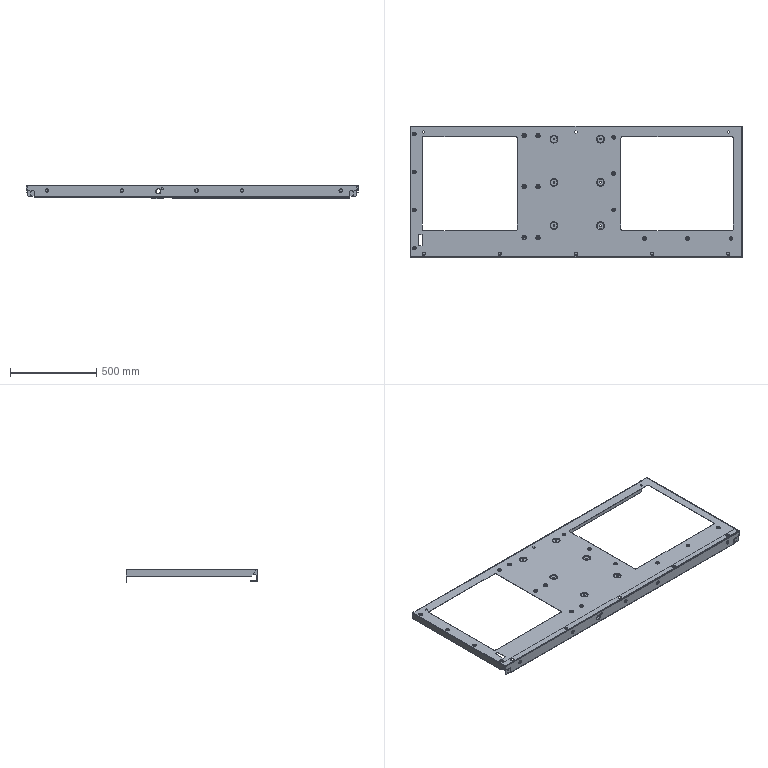Part | STEP file | 1 solid | 795 faces | box 1920 x 759 x 80 mm | volume 2794848 mm3 | plane 391 | cylinder 224 | torus 176 | spline 4 | commonest cylinder face diameters 20.5 x56 7 x33 6.4 x20 4.2 x12 4.7 x12 9 x12